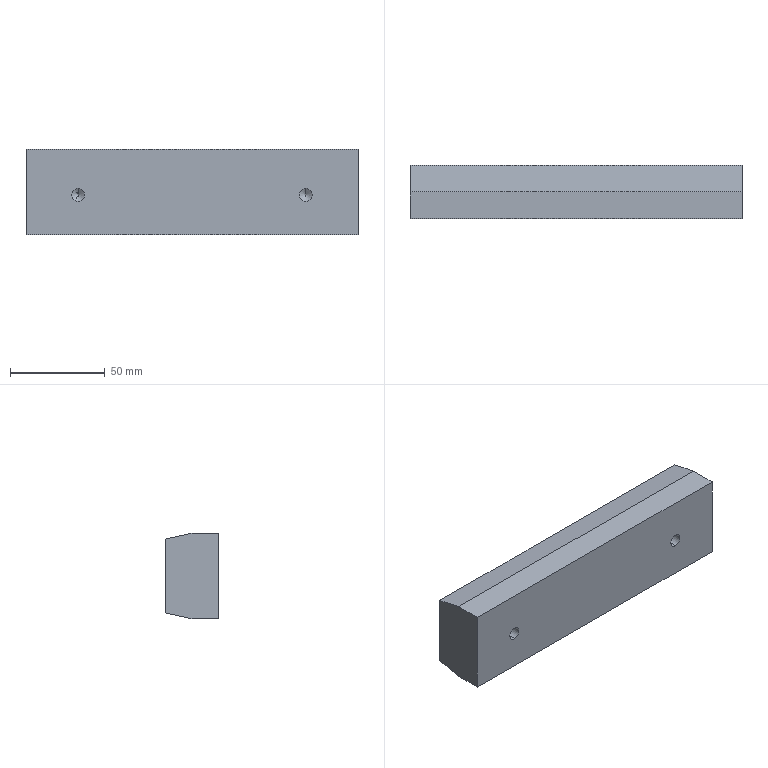Part | SolidWorks | features Extrusion 1, HoleWzd 1, ICE 1 | 1 solid | 16 faces | box 175 x 28 x 45 mm | volume 211666 mm3 | plane 8 | cylinder 4 | cone 4 | commonest cylinder face diameters 6.8 x4
STEP:
#1=CARTESIAN_POINT('',(27.5,-8.25,24.4));
#2=VERTEX_POINT('',#1);
#3=CARTESIAN_POINT('',(27.5,-8.25,17.6));
#4=VERTEX_POINT('',#3);
#5=CARTESIAN_POINT('',(27.5,-8.25,21.));
#6=DIRECTION('',(0.,-1.,0.));
#7=DIRECTION('',(0.,0.,-1.));
#8=AXIS2_PLACEMENT_3D('',#5,#6,#7);
#9=CIRCLE('',#8,3.4);
#10=EDGE_CURVE('',#2,#4,#9,.T.);
#11=ORIENTED_EDGE('',*,*,#10,.F.);
#12=CARTESIAN_POINT('',(27.5,-28.,24.4));
#13=VERTEX_POINT('',#12);
#14=CARTESIAN_POINT('',(27.5,-28.,24.4));
#15=DIRECTION('',(0.,-1.,0.));
#16=VECTOR('',#15,1000.);
#17=LINE('',#14,#16);
#18=EDGE_CURVE('',#2,#13,#17,.T.);
#19=ORIENTED_EDGE('',*,*,#18,.T.);
#20=CARTESIAN_POINT('',(27.5,-28.,17.6));
#21=VERTEX_POINT('',#20);
#22=CARTESIAN_POINT('',(27.5,-28.,21.));
#23=DIRECTION('',(0.,-1.,0.));
#24=DIRECTION('',(0.,0.,-1.));
#25=AXIS2_PLACEMENT_3D('',#22,#23,#24);
#26=CIRCLE('',#25,3.4);
#27=EDGE_CURVE('',#13,#21,#26,.T.);
#28=ORIENTED_EDGE('',*,*,#27,.T.);
#29=CARTESIAN_POINT('',(27.5,-28.,17.6));
#30=DIRECTION('',(0.,-1.,0.));
#31=VECTOR('',#30,1000.);
#32=LINE('',#29,#31);
#33=EDGE_CURVE('',#4,#21,#32,.T.);
#34=ORIENTED_EDGE('',*,*,#33,.F.);
#35=EDGE_LOOP('',(#11,#19,#28,#34));
#36=FACE_OUTER_BOUND('',#35,.T.);
#37=CARTESIAN_POINT('',(27.5,-28.,21.));
#38=DIRECTION('',(0.,-1.,0.));
#39=DIRECTION('',(0.,0.,-1.));
#40=AXIS2_PLACEMENT_3D('',#37,#38,#39);
#41=CYLINDRICAL_SURFACE('',#40,3.4);
#42=ADVANCED_FACE('',(#36),#41,.F.);
#43=CARTESIAN_POINT('',(27.5,-6.207,21.));
#44=VERTEX_POINT('',#43);
#45=CARTESIAN_POINT('',(27.5,-8.25,17.6));
#46=DIRECTION('',(0.,-0.515,-0.8572));
#47=VECTOR('',#46,1000.);
#48=LINE('',#45,#47);
#49=EDGE_CURVE('',#44,#4,#48,.T.);
#50=ORIENTED_EDGE('',*,*,#49,.F.);
#51=CARTESIAN_POINT('',(27.5,-8.25,24.4));
#52=DIRECTION('',(0.,-0.515,0.8572));
#53=VECTOR('',#52,1000.);
#54=LINE('',#51,#53);
#55=EDGE_CURVE('',#44,#2,#54,.T.);
#56=ORIENTED_EDGE('',*,*,#55,.T.);
#57=ORIENTED_EDGE('',*,*,#10,.T.);
#58=EDGE_LOOP('',(#50,#56,#57));
#59=FACE_OUTER_BOUND('',#58,.T.);
#60=CARTESIAN_POINT('',(27.5,-8.25,21.));
#61=DIRECTION('',(0.,-1.,0.));
#62=DIRECTION('',(0.,0.,-1.));
#63=AXIS2_PLACEMENT_3D('',#60,#61,#62);
#64=CONICAL_SURFACE('',#63,3.4,1.03);
#65=ADVANCED_FACE('',(#59),#64,.F.);
#66=CARTESIAN_POINT('',(147.5,-8.25,24.4));
#67=VERTEX_POINT('',#66);
#68=CARTESIAN_POINT('',(147.5,-8.25,17.6));
#69=VERTEX_POINT('',#68);
#70=CARTESIAN_POINT('',(147.5,-8.25,21.));
#71=DIRECTION('',(0.,-1.,0.));
#72=DIRECTION('',(0.,0.,-1.));
#73=AXIS2_PLACEMENT_3D('',#70,#71,#72);
#74=CIRCLE('',#73,3.4);
#75=EDGE_CURVE('',#67,#69,#74,.T.);
#76=ORIENTED_EDGE('',*,*,#75,.F.);
#77=CARTESIAN_POINT('',(147.5,-28.,24.4));
#78=VERTEX_POINT('',#77);
#79=CARTESIAN_POINT('',(147.5,-28.,24.4));
#80=DIRECTION('',(0.,-1.,0.));
#81=VECTOR('',#80,1000.);
#82=LINE('',#79,#81);
#83=EDGE_CURVE('',#67,#78,#82,.T.);
#84=ORIENTED_EDGE('',*,*,#83,.T.);
#85=CARTESIAN_POINT('',(147.5,-28.,17.6));
#86=VERTEX_POINT('',#85);
#87=CARTESIAN_POINT('',(147.5,-28.,21.));
#88=DIRECTION('',(0.,-1.,0.));
#89=DIRECTION('',(0.,0.,-1.));
#90=AXIS2_PLACEMENT_3D('',#87,#88,#89);
#91=CIRCLE('',#90,3.4);
#92=EDGE_CURVE('',#78,#86,#91,.T.);
#93=ORIENTED_EDGE('',*,*,#92,.T.);
#94=CARTESIAN_POINT('',(147.5,-28.,17.6));
#95=DIRECTION('',(0.,-1.,0.));
#96=VECTOR('',#95,1000.);
#97=LINE('',#94,#96);
#98=EDGE_CURVE('',#69,#86,#97,.T.);
#99=ORIENTED_EDGE('',*,*,#98,.F.);
#100=EDGE_LOOP('',(#76,#84,#93,#99));
#101=FACE_OUTER_BOUND('',#100,.T.);
#102=CARTESIAN_POINT('',(147.5,-28.,21.));
#103=DIRECTION('',(0.,-1.,0.));
#104=DIRECTION('',(0.,0.,-1.));
#105=AXIS2_PLACEMENT_3D('',#102,#103,#104);
#106=CYLINDRICAL_SURFACE('',#105,3.4);
#107=ADVANCED_FACE('',(#101),#106,.F.);
#108=CARTESIAN_POINT('',(147.5,-6.207,21.));
#109=VERTEX_POINT('',#108);
#110=CARTESIAN_POINT('',(147.5,-8.25,17.6));
#111=DIRECTION('',(0.,-0.515,-0.8572));
#112=VECTOR('',#111,1000.);
#113=LINE('',#110,#112);
#114=EDGE_CURVE('',#109,#69,#113,.T.);
#115=ORIENTED_EDGE('',*,*,#114,.F.);
#116=CARTESIAN_POINT('',(147.5,-8.25,24.4));
#117=DIRECTION('',(0.,-0.515,0.8572));
#118=VECTOR('',#117,1000.);
#119=LINE('',#116,#118);
#120=EDGE_CURVE('',#109,#67,#119,.T.);
#121=ORIENTED_EDGE('',*,*,#120,.T.);
#122=ORIENTED_EDGE('',*,*,#75,.T.);
#123=EDGE_LOOP('',(#115,#121,#122));
#124=FACE_OUTER_BOUND('',#123,.T.);
#125=CARTESIAN_POINT('',(147.5,-8.25,21.));
#126=DIRECTION('',(0.,-1.,0.));
#127=DIRECTION('',(0.,0.,-1.));
#128=AXIS2_PLACEMENT_3D('',#125,#126,#127);
#129=CONICAL_SURFACE('',#128,3.4,1.03);
#130=ADVANCED_FACE('',(#124),#129,.F.);
#131=CARTESIAN_POINT('',(0.,0.,42.));
#132=VERTEX_POINT('',#131);
#133=CARTESIAN_POINT('',(0.,0.,3.));
#134=VERTEX_POINT('',#133);
#135=CARTESIAN_POINT('',(0.,0.,45.));
#136=DIRECTION('',(0.,0.,-1.));
#137=VECTOR('',#136,1000.);
#138=LINE('',#135,#137);
#139=EDGE_CURVE('',#132,#134,#138,.T.);
#140=ORIENTED_EDGE('',*,*,#139,.T.);
#141=CARTESIAN_POINT('',(0.,-14.,0.));
#142=VERTEX_POINT('',#141);
#143=CARTESIAN_POINT('',(0.,0.,3.));
#144=DIRECTION('',(0.,0.9778,0.2095));
#145=VECTOR('',#144,1000.);
#146=LINE('',#143,#145);
#147=EDGE_CURVE('',#142,#134,#146,.T.);
#148=ORIENTED_EDGE('',*,*,#147,.F.);
#149=CARTESIAN_POINT('',(0.,-28.,0.));
#150=VERTEX_POINT('',#149);
#151=CARTESIAN_POINT('',(0.,0.,0.));
#152=DIRECTION('',(0.,-1.,0.));
#153=VECTOR('',#152,1000.);
#154=LINE('',#151,#153);
#155=EDGE_CURVE('',#142,#150,#154,.T.);
#156=ORIENTED_EDGE('',*,*,#155,.T.);
#157=CARTESIAN_POINT('',(0.,-28.,45.));
#158=VERTEX_POINT('',#157);
#159=CARTESIAN_POINT('',(0.,-28.,45.));
#160=DIRECTION('',(0.,0.,-1.));
#161=VECTOR('',#160,1000.);
#162=LINE('',#159,#161);
#163=EDGE_CURVE('',#158,#150,#162,.T.);
#164=ORIENTED_EDGE('',*,*,#163,.F.);
#165=CARTESIAN_POINT('',(0.,-14.,45.));
#166=VERTEX_POINT('',#165);
#167=CARTESIAN_POINT('',(0.,0.,45.));
#168=DIRECTION('',(0.,-1.,0.));
#169=VECTOR('',#168,1000.);
#170=LINE('',#167,#169);
#171=EDGE_CURVE('',#166,#158,#170,.T.);
#172=ORIENTED_EDGE('',*,*,#171,.F.);
#173=CARTESIAN_POINT('',(0.,0.,42.));
#174=DIRECTION('',(0.,-0.9778,0.2095));
#175=VECTOR('',#174,1000.);
#176=LINE('',#173,#175);
#177=EDGE_CURVE('',#132,#166,#176,.T.);
#178=ORIENTED_EDGE('',*,*,#177,.F.);
#179=EDGE_LOOP('',(#140,#148,#156,#164,#172,#178));
#180=FACE_OUTER_BOUND('',#179,.T.);
#181=CARTESIAN_POINT('',(0.,0.,45.));
#182=DIRECTION('',(1.,0.,0.));
#183=DIRECTION('',(0.,1.,0.));
#184=AXIS2_PLACEMENT_3D('',#181,#182,#183);
#185=PLANE('',#184);
#186=ADVANCED_FACE('',(#180),#185,.F.);
#187=CARTESIAN_POINT('',(27.5,-28.,21.));
#188=DIRECTION('',(0.,-1.,0.));
#189=DIRECTION('',(0.,0.,-1.));
#190=AXIS2_PLACEMENT_3D('',#187,#188,#189);
#191=CIRCLE('',#190,3.4);
#192=EDGE_CURVE('',#21,#13,#191,.T.);
#193=ORIENTED_EDGE('',*,*,#192,.F.);
#194=ORIENTED_EDGE('',*,*,#27,.F.);
#195=EDGE_LOOP('',(#193,#194));
#196=FACE_BOUND('',#195,.T.);
#197=CARTESIAN_POINT('',(147.5,-28.,21.));
#198=DIRECTION('',(0.,-1.,0.));
#199=DIRECTION('',(0.,0.,-1.));
#200=AXIS2_PLACEMENT_3D('',#197,#198,#199);
#201=CIRCLE('',#200,3.4);
#202=EDGE_CURVE('',#86,#78,#201,.T.);
#203=ORIENTED_EDGE('',*,*,#202,.F.);
#204=ORIENTED_EDGE('',*,*,#92,.F.);
#205=EDGE_LOOP('',(#203,#204));
#206=FACE_BOUND('',#205,.T.);
#207=CARTESIAN_POINT('',(175.,-28.,0.));
#208=VERTEX_POINT('',#207);
#209=CARTESIAN_POINT('',(0.,-28.,0.));
#210=DIRECTION('',(1.,0.,0.));
#211=VECTOR('',#210,1000.);
#212=LINE('',#209,#211);
#213=EDGE_CURVE('',#150,#208,#212,.T.);
#214=ORIENTED_EDGE('',*,*,#213,.T.);
#215=CARTESIAN_POINT('',(175.,-28.,45.));
#216=VERTEX_POINT('',#215);
#217=CARTESIAN_POINT('',(175.,-28.,45.));
#218=DIRECTION('',(0.,0.,-1.));
#219=VECTOR('',#218,1000.);
#220=LINE('',#217,#219);
#221=EDGE_CURVE('',#216,#208,#220,.T.);
#222=ORIENTED_EDGE('',*,*,#221,.F.);
#223=CARTESIAN_POINT('',(0.,-28.,45.));
#224=DIRECTION('',(1.,0.,0.));
#225=VECTOR('',#224,1000.);
#226=LINE('',#223,#225);
#227=EDGE_CURVE('',#158,#216,#226,.T.);
#228=ORIENTED_EDGE('',*,*,#227,.F.);
#229=ORIENTED_EDGE('',*,*,#163,.T.);
#230=EDGE_LOOP('',(#214,#222,#228,#229));
#231=FACE_OUTER_BOUND('',#230,.T.);
#232=CARTESIAN_POINT('',(0.,-28.,45.));
#233=DIRECTION('',(0.,1.,0.));
#234=DIRECTION('',(0.,0.,1.));
#235=AXIS2_PLACEMENT_3D('',#232,#233,#234);
#236=PLANE('',#235);
#237=ADVANCED_FACE('',(#196,#206,#231),#236,.F.);
#238=CARTESIAN_POINT('',(175.,-14.,0.));
#239=VERTEX_POINT('',#238);
#240=CARTESIAN_POINT('',(175.,0.,0.));
#241=DIRECTION('',(0.,1.,0.));
#242=VECTOR('',#241,1000.);
#243=LINE('',#240,#242);
#244=EDGE_CURVE('',#208,#239,#243,.T.);
#245=ORIENTED_EDGE('',*,*,#244,.T.);
#246=CARTESIAN_POINT('',(175.,0.,3.));
#247=VERTEX_POINT('',#246);
#248=CARTESIAN_POINT('',(175.,0.,3.));
#249=DIRECTION('',(0.,0.9778,0.2095));
#250=VECTOR('',#249,1000.);
#251=LINE('',#248,#250);
#252=EDGE_CURVE('',#239,#247,#251,.T.);
#253=ORIENTED_EDGE('',*,*,#252,.T.);
#254=CARTESIAN_POINT('',(175.,0.,42.));
#255=VERTEX_POINT('',#254);
#256=CARTESIAN_POINT('',(175.,0.,45.));
#257=DIRECTION('',(0.,0.,-1.));
#258=VECTOR('',#257,1000.);
#259=LINE('',#256,#258);
#260=EDGE_CURVE('',#255,#247,#259,.T.);
#261=ORIENTED_EDGE('',*,*,#260,.F.);
#262=CARTESIAN_POINT('',(175.,-14.,45.));
#263=VERTEX_POINT('',#262);
#264=CARTESIAN_POINT('',(175.,0.,42.));
#265=DIRECTION('',(0.,-0.9778,0.2095));
#266=VECTOR('',#265,1000.);
#267=LINE('',#264,#266);
#268=EDGE_CURVE('',#255,#263,#267,.T.);
#269=ORIENTED_EDGE('',*,*,#268,.T.);
#270=CARTESIAN_POINT('',(175.,0.,45.));
#271=DIRECTION('',(0.,1.,0.));
#272=VECTOR('',#271,1000.);
#273=LINE('',#270,#272);
#274=EDGE_CURVE('',#216,#263,#273,.T.);
#275=ORIENTED_EDGE('',*,*,#274,.F.);
#276=ORIENTED_EDGE('',*,*,#221,.T.);
#277=EDGE_LOOP('',(#245,#253,#261,#269,#275,#276));
#278=FACE_OUTER_BOUND('',#277,.T.);
#279=CARTESIAN_POINT('',(175.,0.,45.));
#280=DIRECTION('',(-1.,0.,0.));
#281=DIRECTION('',(0.,0.,1.));
#282=AXIS2_PLACEMENT_3D('',#279,#280,#281);
#283=PLANE('',#282);
#284=ADVANCED_FACE('',(#278),#283,.F.);
#285=ORIENTED_EDGE('',*,*,#260,.T.);
#286=CARTESIAN_POINT('',(175.,0.,3.));
#287=DIRECTION('',(-1.,0.,0.));
#288=VECTOR('',#287,1000.);
#289=LINE('',#286,#288);
#290=EDGE_CURVE('',#247,#134,#289,.T.);
#291=ORIENTED_EDGE('',*,*,#290,.T.);
#292=ORIENTED_EDGE('',*,*,#139,.F.);
#293=CARTESIAN_POINT('',(175.,0.,42.));
#294=DIRECTION('',(-1.,0.,0.));
#295=VECTOR('',#294,1000.);
#296=LINE('',#293,#295);
#297=EDGE_CURVE('',#255,#132,#296,.T.);
#298=ORIENTED_EDGE('',*,*,#297,.F.);
#299=EDGE_LOOP('',(#285,#291,#292,#298));
#300=FACE_OUTER_BOUND('',#299,.T.);
#301=CARTESIAN_POINT('',(0.,0.,45.));
#302=DIRECTION('',(0.,-1.,0.));
#303=DIRECTION('',(0.,0.,-1.));
#304=AXIS2_PLACEMENT_3D('',#301,#302,#303);
#305=PLANE('',#304);
#306=ADVANCED_FACE('',(#300),#305,.F.);
#307=CARTESIAN_POINT('',(175.,-14.,45.));
#308=DIRECTION('',(-1.,0.,0.));
#309=VECTOR('',#308,1000.);
#310=LINE('',#307,#309);
#311=EDGE_CURVE('',#263,#166,#310,.T.);
#312=ORIENTED_EDGE('',*,*,#311,.T.);
#313=ORIENTED_EDGE('',*,*,#171,.T.);
#314=ORIENTED_EDGE('',*,*,#227,.T.);
#315=ORIENTED_EDGE('',*,*,#274,.T.);
#316=EDGE_LOOP('',(#312,#313,#314,#315));
#317=FACE_OUTER_BOUND('',#316,.T.);
#318=CARTESIAN_POINT('',(0.,0.,45.));
#319=DIRECTION('',(0.,0.,1.));
#320=DIRECTION('',(1.,0.,0.));
#321=AXIS2_PLACEMENT_3D('',#318,#319,#320);
#322=PLANE('',#321);
#323=ADVANCED_FACE('',(#317),#322,.T.);
#324=ORIENTED_EDGE('',*,*,#155,.F.);
#325=CARTESIAN_POINT('',(175.,-14.,0.));
#326=DIRECTION('',(-1.,0.,0.));
#327=VECTOR('',#326,1000.);
#328=LINE('',#325,#327);
#329=EDGE_CURVE('',#239,#142,#328,.T.);
#330=ORIENTED_EDGE('',*,*,#329,.F.);
#331=ORIENTED_EDGE('',*,*,#244,.F.);
#332=ORIENTED_EDGE('',*,*,#213,.F.);
#333=EDGE_LOOP('',(#324,#330,#331,#332));
#334=FACE_OUTER_BOUND('',#333,.T.);
#335=CARTESIAN_POINT('',(0.,0.,0.));
#336=DIRECTION('',(0.,0.,1.));
#337=DIRECTION('',(1.,0.,0.));
#338=AXIS2_PLACEMENT_3D('',#335,#336,#337);
#339=PLANE('',#338);
#340=ADVANCED_FACE('',(#334),#339,.F.);
#341=ORIENTED_EDGE('',*,*,#120,.F.);
#342=ORIENTED_EDGE('',*,*,#114,.T.);
#343=CARTESIAN_POINT('',(147.5,-8.25,21.));
#344=DIRECTION('',(0.,-1.,0.));
#345=DIRECTION('',(0.,0.,-1.));
#346=AXIS2_PLACEMENT_3D('',#343,#344,#345);
#347=CIRCLE('',#346,3.4);
#348=EDGE_CURVE('',#69,#67,#347,.T.);
#349=ORIENTED_EDGE('',*,*,#348,.T.);
#350=EDGE_LOOP('',(#341,#342,#349));
#351=FACE_OUTER_BOUND('',#350,.T.);
#352=CARTESIAN_POINT('',(147.5,-8.25,21.));
#353=DIRECTION('',(0.,-1.,0.));
#354=DIRECTION('',(0.,0.,-1.));
#355=AXIS2_PLACEMENT_3D('',#352,#353,#354);
#356=CONICAL_SURFACE('',#355,3.4,1.03);
#357=ADVANCED_FACE('',(#351),#356,.F.);
#358=ORIENTED_EDGE('',*,*,#83,.F.);
#359=ORIENTED_EDGE('',*,*,#348,.F.);
#360=ORIENTED_EDGE('',*,*,#98,.T.);
#361=ORIENTED_EDGE('',*,*,#202,.T.);
#362=EDGE_LOOP('',(#358,#359,#360,#361));
#363=FACE_OUTER_BOUND('',#362,.T.);
#364=CARTESIAN_POINT('',(147.5,-28.,21.));
#365=DIRECTION('',(0.,-1.,0.));
#366=DIRECTION('',(0.,0.,-1.));
#367=AXIS2_PLACEMENT_3D('',#364,#365,#366);
#368=CYLINDRICAL_SURFACE('',#367,3.4);
#369=ADVANCED_FACE('',(#363),#368,.F.);
#370=ORIENTED_EDGE('',*,*,#55,.F.);
#371=ORIENTED_EDGE('',*,*,#49,.T.);
#372=CARTESIAN_POINT('',(27.5,-8.25,21.));
#373=DIRECTION('',(0.,-1.,0.));
#374=DIRECTION('',(0.,0.,-1.));
#375=AXIS2_PLACEMENT_3D('',#372,#373,#374);
#376=CIRCLE('',#375,3.4);
#377=EDGE_CURVE('',#4,#2,#376,.T.);
#378=ORIENTED_EDGE('',*,*,#377,.T.);
#379=EDGE_LOOP('',(#370,#371,#378));
#380=FACE_OUTER_BOUND('',#379,.T.);
#381=CARTESIAN_POINT('',(27.5,-8.25,21.));
#382=DIRECTION('',(0.,-1.,0.));
#383=DIRECTION('',(0.,0.,-1.));
#384=AXIS2_PLACEMENT_3D('',#381,#382,#383);
#385=CONICAL_SURFACE('',#384,3.4,1.03);
#386=ADVANCED_FACE('',(#380),#385,.F.);
#387=ORIENTED_EDGE('',*,*,#18,.F.);
#388=ORIENTED_EDGE('',*,*,#377,.F.);
#389=ORIENTED_EDGE('',*,*,#33,.T.);
#390=ORIENTED_EDGE('',*,*,#192,.T.);
#391=EDGE_LOOP('',(#387,#388,#389,#390));
#392=FACE_OUTER_BOUND('',#391,.T.);
#393=CARTESIAN_POINT('',(27.5,-28.,21.));
#394=DIRECTION('',(0.,-1.,0.));
#395=DIRECTION('',(0.,0.,-1.));
#396=AXIS2_PLACEMENT_3D('',#393,#394,#395);
#397=CYLINDRICAL_SURFACE('',#396,3.4);
#398=ADVANCED_FACE('',(#392),#397,.F.);
#399=ORIENTED_EDGE('',*,*,#147,.T.);
#400=ORIENTED_EDGE('',*,*,#290,.F.);
#401=ORIENTED_EDGE('',*,*,#252,.F.);
#402=ORIENTED_EDGE('',*,*,#329,.T.);
#403=EDGE_LOOP('',(#399,#400,#401,#402));
#404=FACE_OUTER_BOUND('',#403,.T.);
#405=CARTESIAN_POINT('',(175.,0.,3.));
#406=DIRECTION('',(0.,-0.2095,0.9778));
#407=DIRECTION('',(0.,-0.9778,-0.2095));
#408=AXIS2_PLACEMENT_3D('',#405,#406,#407);
#409=PLANE('',#408);
#410=ADVANCED_FACE('',(#404),#409,.F.);
#411=ORIENTED_EDGE('',*,*,#177,.T.);
#412=ORIENTED_EDGE('',*,*,#311,.F.);
#413=ORIENTED_EDGE('',*,*,#268,.F.);
#414=ORIENTED_EDGE('',*,*,#297,.T.);
#415=EDGE_LOOP('',(#411,#412,#413,#414));
#416=FACE_OUTER_BOUND('',#415,.T.);
#417=CARTESIAN_POINT('',(175.,0.,42.));
#418=DIRECTION('',(0.,-0.2095,-0.9778));
#419=DIRECTION('',(0.,0.9778,-0.2095));
#420=AXIS2_PLACEMENT_3D('',#417,#418,#419);
#421=PLANE('',#420);
#422=ADVANCED_FACE('',(#416),#421,.F.);
#423=CLOSED_SHELL('',(#42,#65,#107,#130,#186,#237,#284,#306,#323,#340,#357,#369,#386,#398,#410,#422));
#424=MANIFOLD_SOLID_BREP('',#423);
#425=CARTESIAN_POINT('',(0.,0.,0.));
#426=DIRECTION('',(0.,0.,1.));
#427=DIRECTION('',(1.,0.,0.));
#428=AXIS2_PLACEMENT_3D('',#425,#426,#427);
#429=(LENGTH_UNIT()NAMED_UNIT(*)SI_UNIT(.MILLI.,.METRE.));
#430=UNCERTAINTY_MEASURE_WITH_UNIT(LENGTH_MEASURE(0.00001),#429,'','');
#431=(NAMED_UNIT(*)PLANE_ANGLE_UNIT()SI_UNIT($,.RADIAN.));
#432=(NAMED_UNIT(*)SI_UNIT($,.STERADIAN.)SOLID_ANGLE_UNIT());
#433=(GEOMETRIC_REPRESENTATION_CONTEXT(3)GLOBAL_UNCERTAINTY_ASSIGNED_CONTEXT((#430))GLOBAL_UNIT_ASSIGNED_CONTEXT((#429,#431,#432))REPRESENTATION_CONTEXT('',''));
#434=ADVANCED_BREP_SHAPE_REPRESENTATION('',(#424,#428),#433);